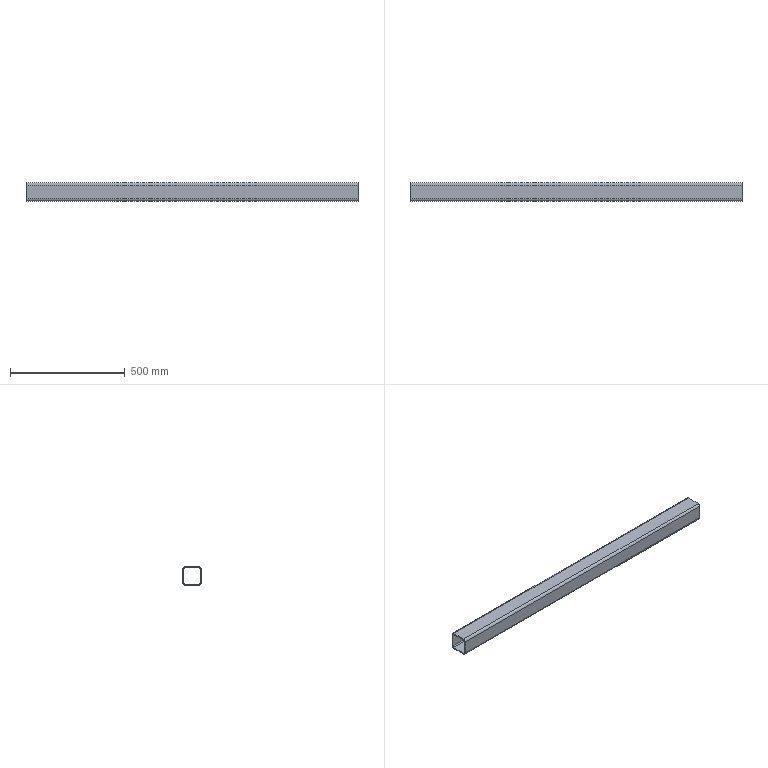Part | SolidWorks | features BaseBody 1 | 1 solid | 18 faces | box 1445 x 80 x 80 mm | volume 2074470 mm3 | plane 10 | cylinder 8 | commonest cylinder face diameters 10 x4 20 x4
STEP:
#1=CARTESIAN_POINT('',(-722.5,30.,-40.));
#2=VERTEX_POINT('',#1);
#3=CARTESIAN_POINT('',(-722.5,40.,-30.));
#4=VERTEX_POINT('',#3);
#5=CARTESIAN_POINT('',(-722.5,30.,-30.));
#6=DIRECTION('',(1.,0.,0.));
#7=DIRECTION('',(0.,0.,-1.));
#8=AXIS2_PLACEMENT_3D('',#5,#6,#7);
#9=CIRCLE('',#8,10.);
#10=EDGE_CURVE('',#2,#4,#9,.T.);
#11=ORIENTED_EDGE('',*,*,#10,.T.);
#12=CARTESIAN_POINT('',(722.5,40.,-30.));
#13=VERTEX_POINT('',#12);
#14=CARTESIAN_POINT('',(722.5,40.,-30.));
#15=DIRECTION('',(-1.,0.,0.));
#16=VECTOR('',#15,1000.);
#17=LINE('',#14,#16);
#18=EDGE_CURVE('',#13,#4,#17,.T.);
#19=ORIENTED_EDGE('',*,*,#18,.F.);
#20=CARTESIAN_POINT('',(722.5,30.,-40.));
#21=VERTEX_POINT('',#20);
#22=CARTESIAN_POINT('',(722.5,30.,-30.));
#23=DIRECTION('',(1.,0.,0.));
#24=DIRECTION('',(0.,0.,-1.));
#25=AXIS2_PLACEMENT_3D('',#22,#23,#24);
#26=CIRCLE('',#25,10.);
#27=EDGE_CURVE('',#21,#13,#26,.T.);
#28=ORIENTED_EDGE('',*,*,#27,.F.);
#29=CARTESIAN_POINT('',(722.5,30.,-40.));
#30=DIRECTION('',(-1.,0.,0.));
#31=VECTOR('',#30,1000.);
#32=LINE('',#29,#31);
#33=EDGE_CURVE('',#21,#2,#32,.T.);
#34=ORIENTED_EDGE('',*,*,#33,.T.);
#35=EDGE_LOOP('',(#11,#19,#28,#34));
#36=FACE_OUTER_BOUND('',#35,.T.);
#37=CARTESIAN_POINT('',(722.5,30.,-30.));
#38=DIRECTION('',(-1.,0.,0.));
#39=DIRECTION('',(0.,0.,1.));
#40=AXIS2_PLACEMENT_3D('',#37,#38,#39);
#41=CYLINDRICAL_SURFACE('',#40,10.);
#42=ADVANCED_FACE('',(#36),#41,.T.);
#43=CARTESIAN_POINT('',(-722.5,40.,30.));
#44=VERTEX_POINT('',#43);
#45=CARTESIAN_POINT('',(-722.5,40.,-30.));
#46=DIRECTION('',(0.,0.,1.));
#47=VECTOR('',#46,1000.);
#48=LINE('',#45,#47);
#49=EDGE_CURVE('',#4,#44,#48,.T.);
#50=ORIENTED_EDGE('',*,*,#49,.T.);
#51=CARTESIAN_POINT('',(722.5,40.,30.));
#52=VERTEX_POINT('',#51);
#53=CARTESIAN_POINT('',(722.5,40.,30.));
#54=DIRECTION('',(-1.,0.,0.));
#55=VECTOR('',#54,1000.);
#56=LINE('',#53,#55);
#57=EDGE_CURVE('',#52,#44,#56,.T.);
#58=ORIENTED_EDGE('',*,*,#57,.F.);
#59=CARTESIAN_POINT('',(722.5,40.,-30.));
#60=DIRECTION('',(0.,0.,1.));
#61=VECTOR('',#60,1000.);
#62=LINE('',#59,#61);
#63=EDGE_CURVE('',#13,#52,#62,.T.);
#64=ORIENTED_EDGE('',*,*,#63,.F.);
#65=ORIENTED_EDGE('',*,*,#18,.T.);
#66=EDGE_LOOP('',(#50,#58,#64,#65));
#67=FACE_OUTER_BOUND('',#66,.T.);
#68=CARTESIAN_POINT('',(722.5,40.,-30.));
#69=DIRECTION('',(0.,-1.,0.));
#70=DIRECTION('',(0.,0.,-1.));
#71=AXIS2_PLACEMENT_3D('',#68,#69,#70);
#72=PLANE('',#71);
#73=ADVANCED_FACE('',(#67),#72,.F.);
#74=CARTESIAN_POINT('',(-722.5,30.,40.));
#75=VERTEX_POINT('',#74);
#76=CARTESIAN_POINT('',(-722.5,30.,30.));
#77=DIRECTION('',(1.,0.,0.));
#78=DIRECTION('',(0.,0.,-1.));
#79=AXIS2_PLACEMENT_3D('',#76,#77,#78);
#80=CIRCLE('',#79,10.);
#81=EDGE_CURVE('',#44,#75,#80,.T.);
#82=ORIENTED_EDGE('',*,*,#81,.T.);
#83=CARTESIAN_POINT('',(722.5,30.,40.));
#84=VERTEX_POINT('',#83);
#85=CARTESIAN_POINT('',(722.5,30.,40.));
#86=DIRECTION('',(-1.,0.,0.));
#87=VECTOR('',#86,1000.);
#88=LINE('',#85,#87);
#89=EDGE_CURVE('',#84,#75,#88,.T.);
#90=ORIENTED_EDGE('',*,*,#89,.F.);
#91=CARTESIAN_POINT('',(722.5,30.,30.));
#92=DIRECTION('',(1.,0.,0.));
#93=DIRECTION('',(0.,0.,-1.));
#94=AXIS2_PLACEMENT_3D('',#91,#92,#93);
#95=CIRCLE('',#94,10.);
#96=EDGE_CURVE('',#52,#84,#95,.T.);
#97=ORIENTED_EDGE('',*,*,#96,.F.);
#98=ORIENTED_EDGE('',*,*,#57,.T.);
#99=EDGE_LOOP('',(#82,#90,#97,#98));
#100=FACE_OUTER_BOUND('',#99,.T.);
#101=CARTESIAN_POINT('',(722.5,30.,30.));
#102=DIRECTION('',(-1.,0.,0.));
#103=DIRECTION('',(0.,0.,1.));
#104=AXIS2_PLACEMENT_3D('',#101,#102,#103);
#105=CYLINDRICAL_SURFACE('',#104,10.);
#106=ADVANCED_FACE('',(#100),#105,.T.);
#107=CARTESIAN_POINT('',(-722.5,-30.,40.));
#108=VERTEX_POINT('',#107);
#109=CARTESIAN_POINT('',(-722.5,-30.,40.));
#110=DIRECTION('',(0.,-1.,0.));
#111=VECTOR('',#110,1000.);
#112=LINE('',#109,#111);
#113=EDGE_CURVE('',#75,#108,#112,.T.);
#114=ORIENTED_EDGE('',*,*,#113,.T.);
#115=CARTESIAN_POINT('',(722.5,-30.,40.));
#116=VERTEX_POINT('',#115);
#117=CARTESIAN_POINT('',(722.5,-30.,40.));
#118=DIRECTION('',(-1.,0.,0.));
#119=VECTOR('',#118,1000.);
#120=LINE('',#117,#119);
#121=EDGE_CURVE('',#116,#108,#120,.T.);
#122=ORIENTED_EDGE('',*,*,#121,.F.);
#123=CARTESIAN_POINT('',(722.5,-30.,40.));
#124=DIRECTION('',(0.,-1.,0.));
#125=VECTOR('',#124,1000.);
#126=LINE('',#123,#125);
#127=EDGE_CURVE('',#84,#116,#126,.T.);
#128=ORIENTED_EDGE('',*,*,#127,.F.);
#129=ORIENTED_EDGE('',*,*,#89,.T.);
#130=EDGE_LOOP('',(#114,#122,#128,#129));
#131=FACE_OUTER_BOUND('',#130,.T.);
#132=CARTESIAN_POINT('',(722.5,-30.,40.));
#133=DIRECTION('',(0.,0.,-1.));
#134=DIRECTION('',(-1.,0.,0.));
#135=AXIS2_PLACEMENT_3D('',#132,#133,#134);
#136=PLANE('',#135);
#137=ADVANCED_FACE('',(#131),#136,.F.);
#138=CARTESIAN_POINT('',(-722.5,-40.,30.));
#139=VERTEX_POINT('',#138);
#140=CARTESIAN_POINT('',(-722.5,-30.,30.));
#141=DIRECTION('',(1.,0.,0.));
#142=DIRECTION('',(0.,0.,-1.));
#143=AXIS2_PLACEMENT_3D('',#140,#141,#142);
#144=CIRCLE('',#143,10.);
#145=EDGE_CURVE('',#108,#139,#144,.T.);
#146=ORIENTED_EDGE('',*,*,#145,.T.);
#147=CARTESIAN_POINT('',(722.5,-40.,30.));
#148=VERTEX_POINT('',#147);
#149=CARTESIAN_POINT('',(722.5,-40.,30.));
#150=DIRECTION('',(-1.,0.,0.));
#151=VECTOR('',#150,1000.);
#152=LINE('',#149,#151);
#153=EDGE_CURVE('',#148,#139,#152,.T.);
#154=ORIENTED_EDGE('',*,*,#153,.F.);
#155=CARTESIAN_POINT('',(722.5,-30.,30.));
#156=DIRECTION('',(1.,0.,0.));
#157=DIRECTION('',(0.,0.,-1.));
#158=AXIS2_PLACEMENT_3D('',#155,#156,#157);
#159=CIRCLE('',#158,10.);
#160=EDGE_CURVE('',#116,#148,#159,.T.);
#161=ORIENTED_EDGE('',*,*,#160,.F.);
#162=ORIENTED_EDGE('',*,*,#121,.T.);
#163=EDGE_LOOP('',(#146,#154,#161,#162));
#164=FACE_OUTER_BOUND('',#163,.T.);
#165=CARTESIAN_POINT('',(722.5,-30.,30.));
#166=DIRECTION('',(-1.,0.,0.));
#167=DIRECTION('',(0.,0.,1.));
#168=AXIS2_PLACEMENT_3D('',#165,#166,#167);
#169=CYLINDRICAL_SURFACE('',#168,10.);
#170=ADVANCED_FACE('',(#164),#169,.T.);
#171=CARTESIAN_POINT('',(-722.5,-40.,-30.));
#172=VERTEX_POINT('',#171);
#173=CARTESIAN_POINT('',(-722.5,-40.,30.));
#174=DIRECTION('',(0.,0.,-1.));
#175=VECTOR('',#174,1000.);
#176=LINE('',#173,#175);
#177=EDGE_CURVE('',#139,#172,#176,.T.);
#178=ORIENTED_EDGE('',*,*,#177,.T.);
#179=CARTESIAN_POINT('',(722.5,-40.,-30.));
#180=VERTEX_POINT('',#179);
#181=CARTESIAN_POINT('',(722.5,-40.,-30.));
#182=DIRECTION('',(-1.,0.,0.));
#183=VECTOR('',#182,1000.);
#184=LINE('',#181,#183);
#185=EDGE_CURVE('',#180,#172,#184,.T.);
#186=ORIENTED_EDGE('',*,*,#185,.F.);
#187=CARTESIAN_POINT('',(722.5,-40.,30.));
#188=DIRECTION('',(0.,0.,-1.));
#189=VECTOR('',#188,1000.);
#190=LINE('',#187,#189);
#191=EDGE_CURVE('',#148,#180,#190,.T.);
#192=ORIENTED_EDGE('',*,*,#191,.F.);
#193=ORIENTED_EDGE('',*,*,#153,.T.);
#194=EDGE_LOOP('',(#178,#186,#192,#193));
#195=FACE_OUTER_BOUND('',#194,.T.);
#196=CARTESIAN_POINT('',(722.5,-40.,30.));
#197=DIRECTION('',(0.,1.,0.));
#198=DIRECTION('',(0.,0.,1.));
#199=AXIS2_PLACEMENT_3D('',#196,#197,#198);
#200=PLANE('',#199);
#201=ADVANCED_FACE('',(#195),#200,.F.);
#202=CARTESIAN_POINT('',(-722.5,-30.,-40.));
#203=VERTEX_POINT('',#202);
#204=CARTESIAN_POINT('',(-722.5,-30.,-30.));
#205=DIRECTION('',(1.,0.,0.));
#206=DIRECTION('',(0.,0.,-1.));
#207=AXIS2_PLACEMENT_3D('',#204,#205,#206);
#208=CIRCLE('',#207,10.);
#209=EDGE_CURVE('',#172,#203,#208,.T.);
#210=ORIENTED_EDGE('',*,*,#209,.T.);
#211=CARTESIAN_POINT('',(722.5,-30.,-40.));
#212=VERTEX_POINT('',#211);
#213=CARTESIAN_POINT('',(722.5,-30.,-40.));
#214=DIRECTION('',(-1.,0.,0.));
#215=VECTOR('',#214,1000.);
#216=LINE('',#213,#215);
#217=EDGE_CURVE('',#212,#203,#216,.T.);
#218=ORIENTED_EDGE('',*,*,#217,.F.);
#219=CARTESIAN_POINT('',(722.5,-30.,-30.));
#220=DIRECTION('',(1.,0.,0.));
#221=DIRECTION('',(0.,0.,-1.));
#222=AXIS2_PLACEMENT_3D('',#219,#220,#221);
#223=CIRCLE('',#222,10.);
#224=EDGE_CURVE('',#180,#212,#223,.T.);
#225=ORIENTED_EDGE('',*,*,#224,.F.);
#226=ORIENTED_EDGE('',*,*,#185,.T.);
#227=EDGE_LOOP('',(#210,#218,#225,#226));
#228=FACE_OUTER_BOUND('',#227,.T.);
#229=CARTESIAN_POINT('',(722.5,-30.,-30.));
#230=DIRECTION('',(-1.,0.,0.));
#231=DIRECTION('',(0.,0.,1.));
#232=AXIS2_PLACEMENT_3D('',#229,#230,#231);
#233=CYLINDRICAL_SURFACE('',#232,10.);
#234=ADVANCED_FACE('',(#228),#233,.T.);
#235=CARTESIAN_POINT('',(-722.5,35.,30.));
#236=VERTEX_POINT('',#235);
#237=CARTESIAN_POINT('',(-722.5,30.,35.));
#238=VERTEX_POINT('',#237);
#239=CARTESIAN_POINT('',(-722.5,30.,30.));
#240=DIRECTION('',(1.,0.,0.));
#241=DIRECTION('',(0.,0.,-1.));
#242=AXIS2_PLACEMENT_3D('',#239,#240,#241);
#243=CIRCLE('',#242,5.);
#244=EDGE_CURVE('',#236,#238,#243,.T.);
#245=ORIENTED_EDGE('',*,*,#244,.F.);
#246=CARTESIAN_POINT('',(722.5,35.,30.));
#247=VERTEX_POINT('',#246);
#248=CARTESIAN_POINT('',(722.5,35.,30.));
#249=DIRECTION('',(-1.,0.,0.));
#250=VECTOR('',#249,1000.);
#251=LINE('',#248,#250);
#252=EDGE_CURVE('',#247,#236,#251,.T.);
#253=ORIENTED_EDGE('',*,*,#252,.F.);
#254=CARTESIAN_POINT('',(722.5,30.,35.));
#255=VERTEX_POINT('',#254);
#256=CARTESIAN_POINT('',(722.5,30.,30.));
#257=DIRECTION('',(1.,0.,0.));
#258=DIRECTION('',(0.,0.,-1.));
#259=AXIS2_PLACEMENT_3D('',#256,#257,#258);
#260=CIRCLE('',#259,5.);
#261=EDGE_CURVE('',#247,#255,#260,.T.);
#262=ORIENTED_EDGE('',*,*,#261,.T.);
#263=CARTESIAN_POINT('',(722.5,30.,35.));
#264=DIRECTION('',(-1.,0.,0.));
#265=VECTOR('',#264,1000.);
#266=LINE('',#263,#265);
#267=EDGE_CURVE('',#255,#238,#266,.T.);
#268=ORIENTED_EDGE('',*,*,#267,.T.);
#269=EDGE_LOOP('',(#245,#253,#262,#268));
#270=FACE_OUTER_BOUND('',#269,.T.);
#271=CARTESIAN_POINT('',(722.5,30.,30.));
#272=DIRECTION('',(-1.,0.,0.));
#273=DIRECTION('',(0.,0.,1.));
#274=AXIS2_PLACEMENT_3D('',#271,#272,#273);
#275=CYLINDRICAL_SURFACE('',#274,5.);
#276=ADVANCED_FACE('',(#270),#275,.F.);
#277=CARTESIAN_POINT('',(-722.5,35.,-30.));
#278=VERTEX_POINT('',#277);
#279=CARTESIAN_POINT('',(-722.5,35.,-30.));
#280=DIRECTION('',(0.,0.,1.));
#281=VECTOR('',#280,1000.);
#282=LINE('',#279,#281);
#283=EDGE_CURVE('',#278,#236,#282,.T.);
#284=ORIENTED_EDGE('',*,*,#283,.F.);
#285=CARTESIAN_POINT('',(722.5,35.,-30.));
#286=VERTEX_POINT('',#285);
#287=CARTESIAN_POINT('',(722.5,35.,-30.));
#288=DIRECTION('',(-1.,0.,0.));
#289=VECTOR('',#288,1000.);
#290=LINE('',#287,#289);
#291=EDGE_CURVE('',#286,#278,#290,.T.);
#292=ORIENTED_EDGE('',*,*,#291,.F.);
#293=CARTESIAN_POINT('',(722.5,35.,-30.));
#294=DIRECTION('',(0.,0.,1.));
#295=VECTOR('',#294,1000.);
#296=LINE('',#293,#295);
#297=EDGE_CURVE('',#286,#247,#296,.T.);
#298=ORIENTED_EDGE('',*,*,#297,.T.);
#299=ORIENTED_EDGE('',*,*,#252,.T.);
#300=EDGE_LOOP('',(#284,#292,#298,#299));
#301=FACE_OUTER_BOUND('',#300,.T.);
#302=CARTESIAN_POINT('',(722.5,35.,-30.));
#303=DIRECTION('',(0.,-1.,0.));
#304=DIRECTION('',(0.,0.,-1.));
#305=AXIS2_PLACEMENT_3D('',#302,#303,#304);
#306=PLANE('',#305);
#307=ADVANCED_FACE('',(#301),#306,.T.);
#308=CARTESIAN_POINT('',(-722.5,30.,-35.));
#309=VERTEX_POINT('',#308);
#310=CARTESIAN_POINT('',(-722.5,30.,-30.));
#311=DIRECTION('',(1.,0.,0.));
#312=DIRECTION('',(0.,0.,-1.));
#313=AXIS2_PLACEMENT_3D('',#310,#311,#312);
#314=CIRCLE('',#313,5.);
#315=EDGE_CURVE('',#309,#278,#314,.T.);
#316=ORIENTED_EDGE('',*,*,#315,.F.);
#317=CARTESIAN_POINT('',(722.5,30.,-35.));
#318=VERTEX_POINT('',#317);
#319=CARTESIAN_POINT('',(722.5,30.,-35.));
#320=DIRECTION('',(-1.,0.,0.));
#321=VECTOR('',#320,1000.);
#322=LINE('',#319,#321);
#323=EDGE_CURVE('',#318,#309,#322,.T.);
#324=ORIENTED_EDGE('',*,*,#323,.F.);
#325=CARTESIAN_POINT('',(722.5,30.,-30.));
#326=DIRECTION('',(1.,0.,0.));
#327=DIRECTION('',(0.,0.,-1.));
#328=AXIS2_PLACEMENT_3D('',#325,#326,#327);
#329=CIRCLE('',#328,5.);
#330=EDGE_CURVE('',#318,#286,#329,.T.);
#331=ORIENTED_EDGE('',*,*,#330,.T.);
#332=ORIENTED_EDGE('',*,*,#291,.T.);
#333=EDGE_LOOP('',(#316,#324,#331,#332));
#334=FACE_OUTER_BOUND('',#333,.T.);
#335=CARTESIAN_POINT('',(722.5,30.,-30.));
#336=DIRECTION('',(-1.,0.,0.));
#337=DIRECTION('',(0.,0.,1.));
#338=AXIS2_PLACEMENT_3D('',#335,#336,#337);
#339=CYLINDRICAL_SURFACE('',#338,5.);
#340=ADVANCED_FACE('',(#334),#339,.F.);
#341=CARTESIAN_POINT('',(-722.5,-30.,-35.));
#342=VERTEX_POINT('',#341);
#343=CARTESIAN_POINT('',(-722.5,30.,-35.));
#344=DIRECTION('',(0.,1.,0.));
#345=VECTOR('',#344,1000.);
#346=LINE('',#343,#345);
#347=EDGE_CURVE('',#342,#309,#346,.T.);
#348=ORIENTED_EDGE('',*,*,#347,.F.);
#349=CARTESIAN_POINT('',(722.5,-30.,-35.));
#350=VERTEX_POINT('',#349);
#351=CARTESIAN_POINT('',(722.5,-30.,-35.));
#352=DIRECTION('',(-1.,0.,0.));
#353=VECTOR('',#352,1000.);
#354=LINE('',#351,#353);
#355=EDGE_CURVE('',#350,#342,#354,.T.);
#356=ORIENTED_EDGE('',*,*,#355,.F.);
#357=CARTESIAN_POINT('',(722.5,30.,-35.));
#358=DIRECTION('',(0.,1.,0.));
#359=VECTOR('',#358,1000.);
#360=LINE('',#357,#359);
#361=EDGE_CURVE('',#350,#318,#360,.T.);
#362=ORIENTED_EDGE('',*,*,#361,.T.);
#363=ORIENTED_EDGE('',*,*,#323,.T.);
#364=EDGE_LOOP('',(#348,#356,#362,#363));
#365=FACE_OUTER_BOUND('',#364,.T.);
#366=CARTESIAN_POINT('',(722.5,30.,-35.));
#367=DIRECTION('',(0.,0.,1.));
#368=DIRECTION('',(1.,0.,0.));
#369=AXIS2_PLACEMENT_3D('',#366,#367,#368);
#370=PLANE('',#369);
#371=ADVANCED_FACE('',(#365),#370,.T.);
#372=CARTESIAN_POINT('',(-722.5,-35.,-30.));
#373=VERTEX_POINT('',#372);
#374=CARTESIAN_POINT('',(-722.5,-30.,-30.));
#375=DIRECTION('',(1.,0.,0.));
#376=DIRECTION('',(0.,0.,-1.));
#377=AXIS2_PLACEMENT_3D('',#374,#375,#376);
#378=CIRCLE('',#377,5.);
#379=EDGE_CURVE('',#373,#342,#378,.T.);
#380=ORIENTED_EDGE('',*,*,#379,.F.);
#381=CARTESIAN_POINT('',(722.5,-35.,-30.));
#382=VERTEX_POINT('',#381);
#383=CARTESIAN_POINT('',(722.5,-35.,-30.));
#384=DIRECTION('',(-1.,0.,0.));
#385=VECTOR('',#384,1000.);
#386=LINE('',#383,#385);
#387=EDGE_CURVE('',#382,#373,#386,.T.);
#388=ORIENTED_EDGE('',*,*,#387,.F.);
#389=CARTESIAN_POINT('',(722.5,-30.,-30.));
#390=DIRECTION('',(1.,0.,0.));
#391=DIRECTION('',(0.,0.,-1.));
#392=AXIS2_PLACEMENT_3D('',#389,#390,#391);
#393=CIRCLE('',#392,5.);
#394=EDGE_CURVE('',#382,#350,#393,.T.);
#395=ORIENTED_EDGE('',*,*,#394,.T.);
#396=ORIENTED_EDGE('',*,*,#355,.T.);
#397=EDGE_LOOP('',(#380,#388,#395,#396));
#398=FACE_OUTER_BOUND('',#397,.T.);
#399=CARTESIAN_POINT('',(722.5,-30.,-30.));
#400=DIRECTION('',(-1.,0.,0.));
#401=DIRECTION('',(0.,0.,1.));
#402=AXIS2_PLACEMENT_3D('',#399,#400,#401);
#403=CYLINDRICAL_SURFACE('',#402,5.);
#404=ADVANCED_FACE('',(#398),#403,.F.);
#405=CARTESIAN_POINT('',(-722.5,-35.,30.));
#406=VERTEX_POINT('',#405);
#407=CARTESIAN_POINT('',(-722.5,-35.,30.));
#408=DIRECTION('',(0.,0.,-1.));
#409=VECTOR('',#408,1000.);
#410=LINE('',#407,#409);
#411=EDGE_CURVE('',#406,#373,#410,.T.);
#412=ORIENTED_EDGE('',*,*,#411,.F.);
#413=CARTESIAN_POINT('',(722.5,-35.,30.));
#414=VERTEX_POINT('',#413);
#415=CARTESIAN_POINT('',(722.5,-35.,30.));
#416=DIRECTION('',(-1.,0.,0.));
#417=VECTOR('',#416,1000.);
#418=LINE('',#415,#417);
#419=EDGE_CURVE('',#414,#406,#418,.T.);
#420=ORIENTED_EDGE('',*,*,#419,.F.);
#421=CARTESIAN_POINT('',(722.5,-35.,30.));
#422=DIRECTION('',(0.,0.,-1.));
#423=VECTOR('',#422,1000.);
#424=LINE('',#421,#423);
#425=EDGE_CURVE('',#414,#382,#424,.T.);
#426=ORIENTED_EDGE('',*,*,#425,.T.);
#427=ORIENTED_EDGE('',*,*,#387,.T.);
#428=EDGE_LOOP('',(#412,#420,#426,#427));
#429=FACE_OUTER_BOUND('',#428,.T.);
#430=CARTESIAN_POINT('',(722.5,-35.,30.));
#431=DIRECTION('',(0.,1.,0.));
#432=DIRECTION('',(0.,0.,1.));
#433=AXIS2_PLACEMENT_3D('',#430,#431,#432);
#434=PLANE('',#433);
#435=ADVANCED_FACE('',(#429),#434,.T.);
#436=CARTESIAN_POINT('',(-722.5,-30.,35.));
#437=VERTEX_POINT('',#436);
#438=CARTESIAN_POINT('',(-722.5,-30.,30.));
#439=DIRECTION('',(1.,0.,0.));
#440=DIRECTION('',(0.,0.,-1.));
#441=AXIS2_PLACEMENT_3D('',#438,#439,#440);
#442=CIRCLE('',#441,5.);
#443=EDGE_CURVE('',#437,#406,#442,.T.);
#444=ORIENTED_EDGE('',*,*,#443,.F.);
#445=CARTESIAN_POINT('',(722.5,-30.,35.));
#446=VERTEX_POINT('',#445);
#447=CARTESIAN_POINT('',(722.5,-30.,35.));
#448=DIRECTION('',(-1.,0.,0.));
#449=VECTOR('',#448,1000.);
#450=LINE('',#447,#449);
#451=EDGE_CURVE('',#446,#437,#450,.T.);
#452=ORIENTED_EDGE('',*,*,#451,.F.);
#453=CARTESIAN_POINT('',(722.5,-30.,30.));
#454=DIRECTION('',(1.,0.,0.));
#455=DIRECTION('',(0.,0.,-1.));
#456=AXIS2_PLACEMENT_3D('',#453,#454,#455);
#457=CIRCLE('',#456,5.);
#458=EDGE_CURVE('',#446,#414,#457,.T.);
#459=ORIENTED_EDGE('',*,*,#458,.T.);
#460=ORIENTED_EDGE('',*,*,#419,.T.);
#461=EDGE_LOOP('',(#444,#452,#459,#460));
#462=FACE_OUTER_BOUND('',#461,.T.);
#463=CARTESIAN_POINT('',(722.5,-30.,30.));
#464=DIRECTION('',(-1.,0.,0.));
#465=DIRECTION('',(0.,0.,1.));
#466=AXIS2_PLACEMENT_3D('',#463,#464,#465);
#467=CYLINDRICAL_SURFACE('',#466,5.);
#468=ADVANCED_FACE('',(#462),#467,.F.);
#469=CARTESIAN_POINT('',(-722.5,-30.,35.));
#470=DIRECTION('',(0.,-1.,0.));
#471=VECTOR('',#470,1000.);
#472=LINE('',#469,#471);
#473=EDGE_CURVE('',#238,#437,#472,.T.);
#474=ORIENTED_EDGE('',*,*,#473,.F.);
#475=ORIENTED_EDGE('',*,*,#267,.F.);
#476=CARTESIAN_POINT('',(722.5,-30.,35.));
#477=DIRECTION('',(0.,-1.,0.));
#478=VECTOR('',#477,1000.);
#479=LINE('',#476,#478);
#480=EDGE_CURVE('',#255,#446,#479,.T.);
#481=ORIENTED_EDGE('',*,*,#480,.T.);
#482=ORIENTED_EDGE('',*,*,#451,.T.);
#483=EDGE_LOOP('',(#474,#475,#481,#482));
#484=FACE_OUTER_BOUND('',#483,.T.);
#485=CARTESIAN_POINT('',(722.5,-30.,35.));
#486=DIRECTION('',(0.,0.,-1.));
#487=DIRECTION('',(-1.,0.,0.));
#488=AXIS2_PLACEMENT_3D('',#485,#486,#487);
#489=PLANE('',#488);
#490=ADVANCED_FACE('',(#484),#489,.T.);
#491=CARTESIAN_POINT('',(-722.5,30.,-40.));
#492=DIRECTION('',(0.,1.,0.));
#493=VECTOR('',#492,1000.);
#494=LINE('',#491,#493);
#495=EDGE_CURVE('',#203,#2,#494,.T.);
#496=ORIENTED_EDGE('',*,*,#495,.T.);
#497=ORIENTED_EDGE('',*,*,#33,.F.);
#498=CARTESIAN_POINT('',(722.5,30.,-40.));
#499=DIRECTION('',(0.,1.,0.));
#500=VECTOR('',#499,1000.);
#501=LINE('',#498,#500);
#502=EDGE_CURVE('',#212,#21,#501,.T.);
#503=ORIENTED_EDGE('',*,*,#502,.F.);
#504=ORIENTED_EDGE('',*,*,#217,.T.);
#505=EDGE_LOOP('',(#496,#497,#503,#504));
#506=FACE_OUTER_BOUND('',#505,.T.);
#507=CARTESIAN_POINT('',(722.5,30.,-40.));
#508=DIRECTION('',(0.,0.,1.));
#509=DIRECTION('',(1.,0.,0.));
#510=AXIS2_PLACEMENT_3D('',#507,#508,#509);
#511=PLANE('',#510);
#512=ADVANCED_FACE('',(#506),#511,.F.);
#513=ORIENTED_EDGE('',*,*,#261,.F.);
#514=ORIENTED_EDGE('',*,*,#297,.F.);
#515=ORIENTED_EDGE('',*,*,#330,.F.);
#516=ORIENTED_EDGE('',*,*,#361,.F.);
#517=ORIENTED_EDGE('',*,*,#394,.F.);
#518=ORIENTED_EDGE('',*,*,#425,.F.);
#519=ORIENTED_EDGE('',*,*,#458,.F.);
#520=ORIENTED_EDGE('',*,*,#480,.F.);
#521=EDGE_LOOP('',(#513,#514,#515,#516,#517,#518,#519,#520));
#522=FACE_BOUND('',#521,.T.);
#523=ORIENTED_EDGE('',*,*,#27,.T.);
#524=ORIENTED_EDGE('',*,*,#63,.T.);
#525=ORIENTED_EDGE('',*,*,#96,.T.);
#526=ORIENTED_EDGE('',*,*,#127,.T.);
#527=ORIENTED_EDGE('',*,*,#160,.T.);
#528=ORIENTED_EDGE('',*,*,#191,.T.);
#529=ORIENTED_EDGE('',*,*,#224,.T.);
#530=ORIENTED_EDGE('',*,*,#502,.T.);
#531=EDGE_LOOP('',(#523,#524,#525,#526,#527,#528,#529,#530));
#532=FACE_OUTER_BOUND('',#531,.T.);
#533=CARTESIAN_POINT('',(722.5,30.,-30.));
#534=DIRECTION('',(1.,0.,0.));
#535=DIRECTION('',(0.,0.,-1.));
#536=AXIS2_PLACEMENT_3D('',#533,#534,#535);
#537=PLANE('',#536);
#538=ADVANCED_FACE('',(#522,#532),#537,.T.);
#539=ORIENTED_EDGE('',*,*,#244,.T.);
#540=ORIENTED_EDGE('',*,*,#473,.T.);
#541=ORIENTED_EDGE('',*,*,#443,.T.);
#542=ORIENTED_EDGE('',*,*,#411,.T.);
#543=ORIENTED_EDGE('',*,*,#379,.T.);
#544=ORIENTED_EDGE('',*,*,#347,.T.);
#545=ORIENTED_EDGE('',*,*,#315,.T.);
#546=ORIENTED_EDGE('',*,*,#283,.T.);
#547=EDGE_LOOP('',(#539,#540,#541,#542,#543,#544,#545,#546));
#548=FACE_BOUND('',#547,.T.);
#549=ORIENTED_EDGE('',*,*,#10,.F.);
#550=ORIENTED_EDGE('',*,*,#495,.F.);
#551=ORIENTED_EDGE('',*,*,#209,.F.);
#552=ORIENTED_EDGE('',*,*,#177,.F.);
#553=ORIENTED_EDGE('',*,*,#145,.F.);
#554=ORIENTED_EDGE('',*,*,#113,.F.);
#555=ORIENTED_EDGE('',*,*,#81,.F.);
#556=ORIENTED_EDGE('',*,*,#49,.F.);
#557=EDGE_LOOP('',(#549,#550,#551,#552,#553,#554,#555,#556));
#558=FACE_OUTER_BOUND('',#557,.T.);
#559=CARTESIAN_POINT('',(-722.5,30.,-30.));
#560=DIRECTION('',(1.,0.,0.));
#561=DIRECTION('',(0.,0.,-1.));
#562=AXIS2_PLACEMENT_3D('',#559,#560,#561);
#563=PLANE('',#562);
#564=ADVANCED_FACE('',(#548,#558),#563,.F.);
#565=CLOSED_SHELL('',(#42,#73,#106,#137,#170,#201,#234,#276,#307,#340,#371,#404,#435,#468,#490,#512,#538,#564));
#566=MANIFOLD_SOLID_BREP('',#565);
#567=CARTESIAN_POINT('',(0.,0.,0.));
#568=DIRECTION('',(0.,0.,1.));
#569=DIRECTION('',(1.,0.,0.));
#570=AXIS2_PLACEMENT_3D('',#567,#568,#569);
#571=(LENGTH_UNIT()NAMED_UNIT(*)SI_UNIT(.MILLI.,.METRE.));
#572=UNCERTAINTY_MEASURE_WITH_UNIT(LENGTH_MEASURE(0.00001),#571,'','');
#573=(NAMED_UNIT(*)PLANE_ANGLE_UNIT()SI_UNIT($,.RADIAN.));
#574=(NAMED_UNIT(*)SI_UNIT($,.STERADIAN.)SOLID_ANGLE_UNIT());
#575=(GEOMETRIC_REPRESENTATION_CONTEXT(3)GLOBAL_UNCERTAINTY_ASSIGNED_CONTEXT((#572))GLOBAL_UNIT_ASSIGNED_CONTEXT((#571,#573,#574))REPRESENTATION_CONTEXT('',''));
#576=ADVANCED_BREP_SHAPE_REPRESENTATION('',(#566,#570),#575);